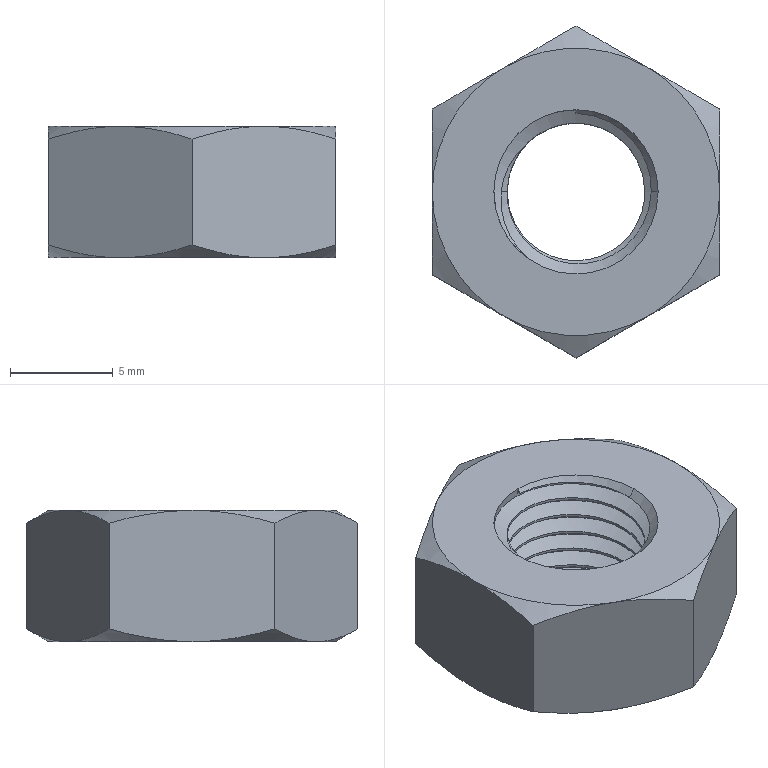Part | SolidWorks | features ICE 4, CombineBodies 1, Extrusion 1, Helix 1, MirrorPattern 1, Scale 1, SweepCut 1 | 1 solid | 55 faces | box 14 x 16.166 x 6.4 mm | volume 804.072 mm3 | cylinder 26 | cone 18 | plane 9 | spline 2 | commonest cylinder face diameters 8 x14 6.701 x12